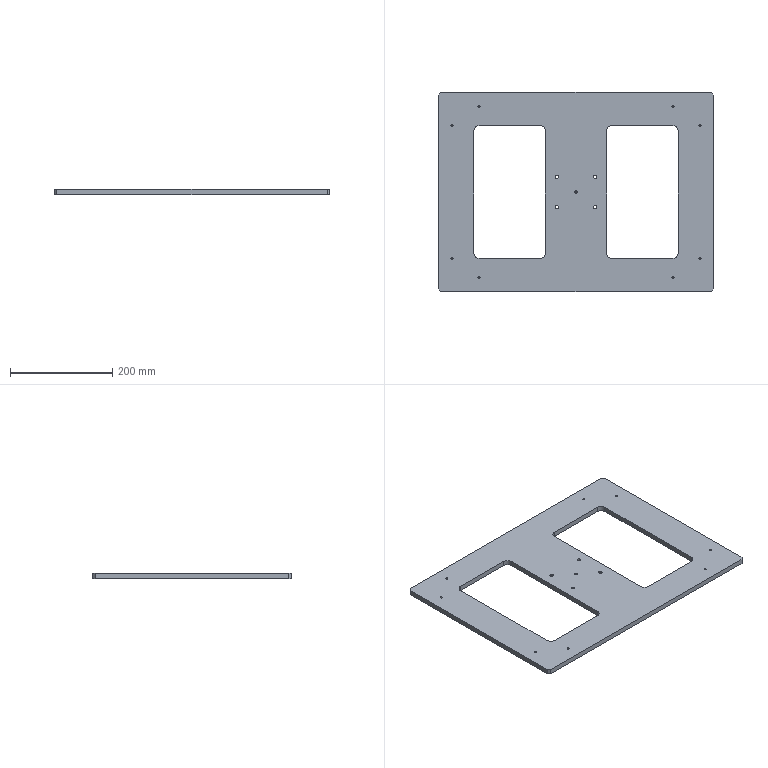CAM job | NX | 3-axis milling, drilling | part box 540 x 390 x 10 mm | stock box 545 x 395 x 10 mm
Tools:
number,name,description,diameter,corner_radius,flute_length,length,flutes
6,D6,平底铣刀-粗,6.0,0.0,25.0,75.0,2
9,D10,平底铣刀-粗,10.0,0.0,35.0,75.0,2
11,D3-J,平底铣刀-精,3.0,0.0,50.0,75.0,2
7,D6-J,平底铣刀-精,6.0,0.0,25.0,75.0,2
2,D6倒角刀,倒角刀,6.0,0.0,3.0,25.0,2
14,ZT4.2,钻头,4.2,0.0,35.0,50.0,2
15,ZT5,钻头,5.0,0.0,35.0,50.0,2
17,ZT6.6,钻头,6.6,0.0,35.0,50.0,2
Operations:
program,operation,operation_type,tool,method,geometry_group,spindle_rpm,surface_speed,feed_per_tooth,feed_cut,feed_plunge,cut_length_mm,path_length_mm,cut_time_min,machine_time_min
B,DRILLCHAMFER_2,Operation,D6倒角刀,METHOD,W-B,8000.0,150.796,0.0625,1000.0,0.0,42.936,1308.054,0.0429,0.1694
B,DRILLCHAMFER_3,Operation,D6倒角刀,METHOD,W-B,8000.0,150.796,0.0625,1000.0,0.0,5.8,51.6,0.0058,0.0104
B,C0.3封闭铣廓倒角6X45L_COPY,PlanarMilling,D6倒角刀,爬面_倒角-切深0-步距G,W-B,7000.0,131.0,0.1071,1500.0,100.0,3449.146,3993.049,2.299,2.354
B,C0.3封闭铣廓倒角6X45L_COPY_1,PlanarMilling,D6倒角刀,爬面_倒角-切深0-步距G,W-B,7000.0,131.0,0.1071,1500.0,100.0,118.278,462.42,0.0789,0.1133
A,打点,Operation,D6倒角刀,METHOD,W-A,3000.0,56.549,0.0333,200.0,0.0,32.5,1525.324,0.1625,0.3118
A,DRILLING,Operation,ZT4.2,METHOD,W-A,3000.0,38.924,0.0167,100.0,0.0,85.6,1379.096,0.856,0.9853
A,DRILLING_2,Operation,ZT5,METHOD,W-A,2800.0,43.982,0.0214,120.0,0.0,10.7,61.4,0.0892,0.0942
A,DRILLING_3,Operation,ZT6.6,METHOD,W-A,2500.0,51.836,0.03,150.0,0.0,42.8,323.623,0.2853,0.3134
A,POCKETROUGHING_1,VolumeBased25DMillingOperation,D10,METHOD,W-A,6000.0,188.0,0.25,4000.0,80.0,31536.086,32021.887,7.884,7.933
A,外形粗_2,VolumeBased25DMillingOperation,D10,METHOD,W-A,6000.0,188.0,0.25,4000.0,80.0,39488.4,39536.4,9.872,9.877
A,孔粗_1,CylinderMilling,D6,METHOD,W-A,6000.0,113.097,0.1667,2000.0,100.0,947.472,1328.472,0.4737,0.5118
A,POCKETSEMI-FINISH_1,VolumeBased25DMillingOperation,D6-J,METHOD,W-A,6000.0,113.0,0.0833,1000.0,100.0,1538.216,2113.177,1.538,1.596
A,框精_1,VolumeBased25DMillingOperation,D6-J,METHOD,W-A,6000.0,113.0,0.0833,1000.0,100.0,1537.816,2114.147,1.538,1.595
A,孔侧_1,CylinderMilling,D6-J,METHOD,W-A,6000.0,113.097,0.0667,800.0,100.0,86.767,496.167,0.1085,0.1494
A,底壁铣螺旋精光-中_COPY,VolumeBased25DMillingOperation,D3-J,螺旋精光-切深K-步距G,W-A,8000.0,75.396,0.0375,600.0,100.0,1061.336,2610.908,1.769,1.924
A,底壁铣螺旋精光-中_COPY_COPY,VolumeBased25DMillingOperation,D3-J,螺旋精光-切深K-步距G,W-A,8000.0,75.398,0.0187,300.0,100.0,227.126,275.426,0.7571,0.7619
A,底壁铣螺旋精光-中_COPY_COPY_COPY,VolumeBased25DMillingOperation,D3-J,螺旋精光-切深K-步距G,W-A,8000.0,75.398,0.0312,500.0,100.0,545.08,965.112,1.09,1.132
A,仅选体,SurfaceContour,D6倒角刀,METHOD,W-A,6000.0,113.0,0.125,1200.0,100.0,3433.207,3871.238,2.861,2.905
A,DRILLCHAMFER_1,Operation,D6倒角刀,METHOD,W-A,5000.0,94.248,0.015,150.0,0.0,42.936,1308.054,0.2862,0.4128
A,MILLCHAMFER_1,PlanarMilling,D6倒角刀,METHOD,W-A,6000.0,113.097,0.05,600.0,100.0,10.327,52.527,0.0172,0.0214
A,MILLCHAMFER_2,PlanarMilling,D6倒角刀,METHOD,W-A,6000.0,113.097,0.05,600.0,100.0,139.642,506.837,0.2327,0.2695
A,PROFILESEMI-FINISH_2,VolumeBased25DMillingOperation,D6-J,METHOD,W-A,6000.0,113.0,0.0833,1000.0,100.0,1872.05,1930.05,1.872,1.878
A,外形精_2,VolumeBased25DMillingOperation,D6-J,METHOD,W-A,6000.0,113.0,0.0833,1000.0,100.0,1871.85,1930.45,1.872,1.878